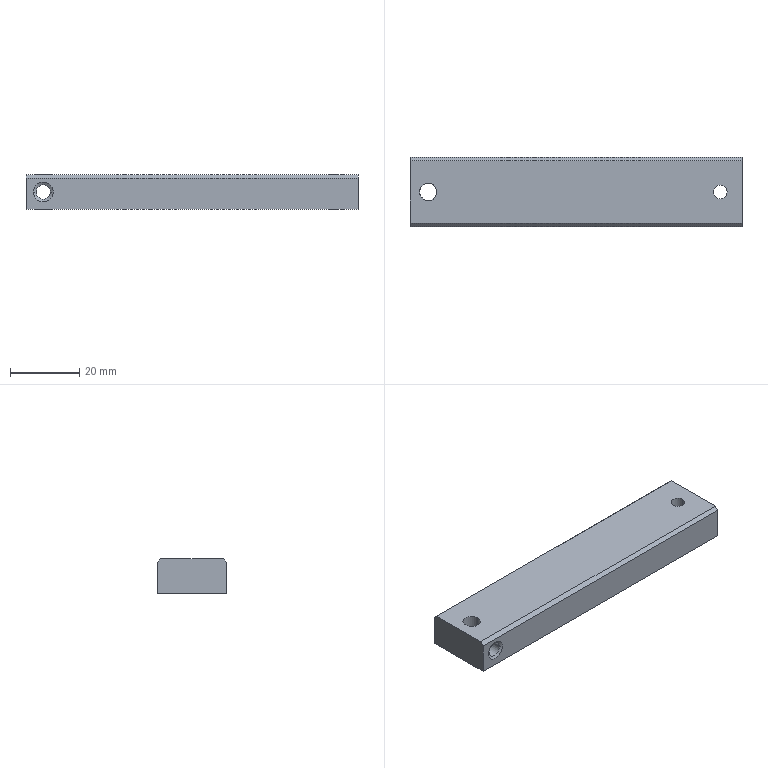Part | NX | 1 solid | 24 faces | box 96 x 20 x 10 mm | volume 18522 mm3 | cylinder 10 | plane 8 | cone 6 | commonest cylinder face diameters 4.2 x4 3.3 x2 4 x2 5 x2
STEP:
#1=CARTESIAN_POINT('',(-48.,-10.,-5.));
#2=VERTEX_POINT('',#1);
#3=CARTESIAN_POINT('',(-48.,10.,-5.));
#4=VERTEX_POINT('',#3);
#5=CARTESIAN_POINT('',(-48.,-10.,-5.));
#6=DIRECTION('',(0.,1.,0.));
#7=VECTOR('',#6,1000.);
#8=LINE('',#5,#7);
#9=EDGE_CURVE('',#2,#4,#8,.T.);
#10=ORIENTED_EDGE('',*,*,#9,.T.);
#11=CARTESIAN_POINT('',(48.,10.,-5.));
#12=VERTEX_POINT('',#11);
#13=CARTESIAN_POINT('',(0.,10.,-5.));
#14=DIRECTION('',(-1.,0.,0.));
#15=VECTOR('',#14,1000.);
#16=LINE('',#13,#15);
#17=EDGE_CURVE('',#12,#4,#16,.T.);
#18=ORIENTED_EDGE('',*,*,#17,.F.);
#19=CARTESIAN_POINT('',(48.,-10.,-5.));
#20=VERTEX_POINT('',#19);
#21=CARTESIAN_POINT('',(48.,0.,-5.));
#22=DIRECTION('',(0.,1.,0.));
#23=VECTOR('',#22,1000.);
#24=LINE('',#21,#23);
#25=EDGE_CURVE('',#20,#12,#24,.T.);
#26=ORIENTED_EDGE('',*,*,#25,.F.);
#27=CARTESIAN_POINT('',(0.,-10.,-5.));
#28=DIRECTION('',(1.,0.,0.));
#29=VECTOR('',#28,1000.);
#30=LINE('',#27,#29);
#31=EDGE_CURVE('',#2,#20,#30,.T.);
#32=ORIENTED_EDGE('',*,*,#31,.F.);
#33=EDGE_LOOP('',(#10,#18,#26,#32));
#34=FACE_BOUND('',#33,.T.);
#35=CARTESIAN_POINT('',(-45.2,0.,-5.));
#36=VERTEX_POINT('',#35);
#37=CARTESIAN_POINT('',(-40.2,0.,-5.));
#38=VERTEX_POINT('',#37);
#39=CARTESIAN_POINT('',(-42.7,0.,-5.));
#40=DIRECTION('',(0.,0.,1.));
#41=DIRECTION('',(-1.,0.,0.));
#42=AXIS2_PLACEMENT_3D('',#39,#40,#41);
#43=CIRCLE('',#42,2.5);
#44=EDGE_CURVE('',#36,#38,#43,.T.);
#45=ORIENTED_EDGE('',*,*,#44,.T.);
#46=CARTESIAN_POINT('',(-42.7,0.,-5.));
#47=DIRECTION('',(0.,0.,1.));
#48=DIRECTION('',(-1.,0.,0.));
#49=AXIS2_PLACEMENT_3D('',#46,#47,#48);
#50=CIRCLE('',#49,2.5);
#51=EDGE_CURVE('',#38,#36,#50,.T.);
#52=ORIENTED_EDGE('',*,*,#51,.T.);
#53=EDGE_LOOP('',(#45,#52));
#54=FACE_BOUND('',#53,.T.);
#55=CARTESIAN_POINT('',(43.7,0.,-5.));
#56=VERTEX_POINT('',#55);
#57=CARTESIAN_POINT('',(39.7,0.,-5.));
#58=VERTEX_POINT('',#57);
#59=CARTESIAN_POINT('',(41.7,0.,-5.));
#60=DIRECTION('',(0.,0.,-1.));
#61=DIRECTION('',(-1.,0.,0.));
#62=AXIS2_PLACEMENT_3D('',#59,#60,#61);
#63=CIRCLE('',#62,2.);
#64=EDGE_CURVE('',#56,#58,#63,.T.);
#65=ORIENTED_EDGE('',*,*,#64,.F.);
#66=CARTESIAN_POINT('',(41.7,0.,-5.));
#67=DIRECTION('',(0.,0.,-1.));
#68=DIRECTION('',(-1.,0.,0.));
#69=AXIS2_PLACEMENT_3D('',#66,#67,#68);
#70=CIRCLE('',#69,2.);
#71=EDGE_CURVE('',#58,#56,#70,.T.);
#72=ORIENTED_EDGE('',*,*,#71,.F.);
#73=EDGE_LOOP('',(#65,#72));
#74=FACE_BOUND('',#73,.T.);
#75=CARTESIAN_POINT('',(0.,0.,-5.));
#76=DIRECTION('',(0.,0.,1.));
#77=DIRECTION('',(1.,0.,0.));
#78=AXIS2_PLACEMENT_3D('',#75,#76,#77);
#79=PLANE('',#78);
#80=ADVANCED_FACE('',(#34,#54,#74),#79,.F.);
#81=ORIENTED_EDGE('',*,*,#9,.F.);
#82=CARTESIAN_POINT('',(-48.,-10.,4.));
#83=VERTEX_POINT('',#82);
#84=CARTESIAN_POINT('',(-48.,-10.,0.));
#85=DIRECTION('',(0.,0.,1.));
#86=VECTOR('',#85,1000.);
#87=LINE('',#84,#86);
#88=EDGE_CURVE('',#2,#83,#87,.T.);
#89=ORIENTED_EDGE('',*,*,#88,.T.);
#90=CARTESIAN_POINT('',(-48.,-9.,5.));
#91=VERTEX_POINT('',#90);
#92=CARTESIAN_POINT('',(-48.,-9.,5.));
#93=DIRECTION('',(0.,-0.7071,-0.7071));
#94=VECTOR('',#93,1000.);
#95=LINE('',#92,#94);
#96=EDGE_CURVE('',#91,#83,#95,.T.);
#97=ORIENTED_EDGE('',*,*,#96,.F.);
#98=CARTESIAN_POINT('',(-48.,9.,5.));
#99=VERTEX_POINT('',#98);
#100=CARTESIAN_POINT('',(-48.,-9.,5.));
#101=DIRECTION('',(0.,1.,0.));
#102=VECTOR('',#101,1000.);
#103=LINE('',#100,#102);
#104=EDGE_CURVE('',#91,#99,#103,.T.);
#105=ORIENTED_EDGE('',*,*,#104,.T.);
#106=CARTESIAN_POINT('',(-48.,10.,4.));
#107=VERTEX_POINT('',#106);
#108=CARTESIAN_POINT('',(-48.,10.,4.));
#109=DIRECTION('',(0.,-0.7071,0.7071));
#110=VECTOR('',#109,1000.);
#111=LINE('',#108,#110);
#112=EDGE_CURVE('',#107,#99,#111,.T.);
#113=ORIENTED_EDGE('',*,*,#112,.F.);
#114=CARTESIAN_POINT('',(-48.,10.,0.));
#115=DIRECTION('',(0.,0.,-1.));
#116=VECTOR('',#115,1000.);
#117=LINE('',#114,#116);
#118=EDGE_CURVE('',#107,#4,#117,.T.);
#119=ORIENTED_EDGE('',*,*,#118,.T.);
#120=EDGE_LOOP('',(#81,#89,#97,#105,#113,#119));
#121=FACE_BOUND('',#120,.T.);
#122=CARTESIAN_POINT('',(-48.,10.,-5.));
#123=DIRECTION('',(-1.,0.,0.));
#124=DIRECTION('',(0.,0.,1.));
#125=AXIS2_PLACEMENT_3D('',#122,#123,#124);
#126=PLANE('',#125);
#127=ADVANCED_FACE('',(#121),#126,.T.);
#128=ORIENTED_EDGE('',*,*,#17,.T.);
#129=ORIENTED_EDGE('',*,*,#118,.F.);
#130=CARTESIAN_POINT('',(48.,10.,4.));
#131=VERTEX_POINT('',#130);
#132=CARTESIAN_POINT('',(0.,10.,4.));
#133=DIRECTION('',(1.,0.,0.));
#134=VECTOR('',#133,1000.);
#135=LINE('',#132,#134);
#136=EDGE_CURVE('',#107,#131,#135,.T.);
#137=ORIENTED_EDGE('',*,*,#136,.T.);
#138=CARTESIAN_POINT('',(48.,10.,0.));
#139=DIRECTION('',(0.,0.,-1.));
#140=VECTOR('',#139,1000.);
#141=LINE('',#138,#140);
#142=EDGE_CURVE('',#131,#12,#141,.T.);
#143=ORIENTED_EDGE('',*,*,#142,.T.);
#144=EDGE_LOOP('',(#128,#129,#137,#143));
#145=FACE_BOUND('',#144,.T.);
#146=CARTESIAN_POINT('',(-40.14,10.,0.));
#147=VERTEX_POINT('',#146);
#148=CARTESIAN_POINT('',(-45.86,10.,0.));
#149=VERTEX_POINT('',#148);
#150=CARTESIAN_POINT('',(-43.,10.,0.));
#151=DIRECTION('',(0.,1.,0.));
#152=DIRECTION('',(1.,0.,0.));
#153=AXIS2_PLACEMENT_3D('',#150,#151,#152);
#154=CIRCLE('',#153,2.86);
#155=EDGE_CURVE('',#147,#149,#154,.T.);
#156=ORIENTED_EDGE('',*,*,#155,.F.);
#157=CARTESIAN_POINT('',(-43.,10.,0.));
#158=DIRECTION('',(0.,1.,0.));
#159=DIRECTION('',(1.,0.,0.));
#160=AXIS2_PLACEMENT_3D('',#157,#158,#159);
#161=CIRCLE('',#160,2.86);
#162=EDGE_CURVE('',#149,#147,#161,.T.);
#163=ORIENTED_EDGE('',*,*,#162,.F.);
#164=EDGE_LOOP('',(#156,#163));
#165=FACE_BOUND('',#164,.T.);
#166=CARTESIAN_POINT('',(48.,10.,-5.));
#167=DIRECTION('',(0.,1.,0.));
#168=DIRECTION('',(1.,0.,0.));
#169=AXIS2_PLACEMENT_3D('',#166,#167,#168);
#170=PLANE('',#169);
#171=ADVANCED_FACE('',(#145,#165),#170,.T.);
#172=ORIENTED_EDGE('',*,*,#25,.T.);
#173=ORIENTED_EDGE('',*,*,#142,.F.);
#174=CARTESIAN_POINT('',(48.,9.,5.));
#175=VERTEX_POINT('',#174);
#176=CARTESIAN_POINT('',(48.,14.,0.));
#177=DIRECTION('',(0.,-0.7071,0.7071));
#178=VECTOR('',#177,1000.);
#179=LINE('',#176,#178);
#180=EDGE_CURVE('',#131,#175,#179,.T.);
#181=ORIENTED_EDGE('',*,*,#180,.T.);
#182=CARTESIAN_POINT('',(48.,-9.,5.));
#183=VERTEX_POINT('',#182);
#184=CARTESIAN_POINT('',(48.,0.,5.));
#185=DIRECTION('',(0.,1.,0.));
#186=VECTOR('',#185,1000.);
#187=LINE('',#184,#186);
#188=EDGE_CURVE('',#183,#175,#187,.T.);
#189=ORIENTED_EDGE('',*,*,#188,.F.);
#190=CARTESIAN_POINT('',(48.,-10.,4.));
#191=VERTEX_POINT('',#190);
#192=CARTESIAN_POINT('',(48.,-14.,0.));
#193=DIRECTION('',(0.,-0.7071,-0.7071));
#194=VECTOR('',#193,1000.);
#195=LINE('',#192,#194);
#196=EDGE_CURVE('',#183,#191,#195,.T.);
#197=ORIENTED_EDGE('',*,*,#196,.T.);
#198=CARTESIAN_POINT('',(48.,-10.,0.));
#199=DIRECTION('',(0.,0.,1.));
#200=VECTOR('',#199,1000.);
#201=LINE('',#198,#200);
#202=EDGE_CURVE('',#20,#191,#201,.T.);
#203=ORIENTED_EDGE('',*,*,#202,.F.);
#204=EDGE_LOOP('',(#172,#173,#181,#189,#197,#203));
#205=FACE_BOUND('',#204,.T.);
#206=CARTESIAN_POINT('',(48.,-2.315,0.));
#207=VERTEX_POINT('',#206);
#208=CARTESIAN_POINT('',(48.,2.315,0.));
#209=VERTEX_POINT('',#208);
#210=CARTESIAN_POINT('',(48.,0.,0.));
#211=DIRECTION('',(1.,0.,0.));
#212=DIRECTION('',(0.,-1.,0.));
#213=AXIS2_PLACEMENT_3D('',#210,#211,#212);
#214=CIRCLE('',#213,2.315);
#215=EDGE_CURVE('',#207,#209,#214,.T.);
#216=ORIENTED_EDGE('',*,*,#215,.F.);
#217=CARTESIAN_POINT('',(48.,0.,0.));
#218=DIRECTION('',(1.,0.,0.));
#219=DIRECTION('',(0.,-1.,0.));
#220=AXIS2_PLACEMENT_3D('',#217,#218,#219);
#221=CIRCLE('',#220,2.315);
#222=EDGE_CURVE('',#209,#207,#221,.T.);
#223=ORIENTED_EDGE('',*,*,#222,.F.);
#224=EDGE_LOOP('',(#216,#223));
#225=FACE_BOUND('',#224,.T.);
#226=CARTESIAN_POINT('',(48.,-10.,-5.));
#227=DIRECTION('',(1.,0.,0.));
#228=DIRECTION('',(0.,1.,0.));
#229=AXIS2_PLACEMENT_3D('',#226,#227,#228);
#230=PLANE('',#229);
#231=ADVANCED_FACE('',(#205,#225),#230,.T.);
#232=ORIENTED_EDGE('',*,*,#31,.T.);
#233=ORIENTED_EDGE('',*,*,#202,.T.);
#234=CARTESIAN_POINT('',(0.,-10.,4.));
#235=DIRECTION('',(-1.,0.,0.));
#236=VECTOR('',#235,1000.);
#237=LINE('',#234,#236);
#238=EDGE_CURVE('',#191,#83,#237,.T.);
#239=ORIENTED_EDGE('',*,*,#238,.T.);
#240=ORIENTED_EDGE('',*,*,#88,.F.);
#241=EDGE_LOOP('',(#232,#233,#239,#240));
#242=FACE_BOUND('',#241,.T.);
#243=CARTESIAN_POINT('',(-40.14,-10.,0.));
#244=VERTEX_POINT('',#243);
#245=CARTESIAN_POINT('',(-45.86,-10.,0.));
#246=VERTEX_POINT('',#245);
#247=CARTESIAN_POINT('',(-43.,-10.,0.));
#248=DIRECTION('',(0.,-1.,0.));
#249=DIRECTION('',(-1.,0.,0.));
#250=AXIS2_PLACEMENT_3D('',#247,#248,#249);
#251=CIRCLE('',#250,2.86);
#252=EDGE_CURVE('',#244,#246,#251,.T.);
#253=ORIENTED_EDGE('',*,*,#252,.F.);
#254=CARTESIAN_POINT('',(-43.,-10.,0.));
#255=DIRECTION('',(0.,-1.,0.));
#256=DIRECTION('',(-1.,0.,0.));
#257=AXIS2_PLACEMENT_3D('',#254,#255,#256);
#258=CIRCLE('',#257,2.86);
#259=EDGE_CURVE('',#246,#244,#258,.T.);
#260=ORIENTED_EDGE('',*,*,#259,.F.);
#261=EDGE_LOOP('',(#253,#260));
#262=FACE_BOUND('',#261,.T.);
#263=CARTESIAN_POINT('',(-48.,-10.,-5.));
#264=DIRECTION('',(0.,-1.,0.));
#265=DIRECTION('',(0.,0.,-1.));
#266=AXIS2_PLACEMENT_3D('',#263,#264,#265);
#267=PLANE('',#266);
#268=ADVANCED_FACE('',(#242,#262),#267,.T.);
#269=CARTESIAN_POINT('',(48.,-9.,5.));
#270=DIRECTION('',(-1.,0.,0.));
#271=VECTOR('',#270,1000.);
#272=LINE('',#269,#271);
#273=EDGE_CURVE('',#183,#91,#272,.T.);
#274=ORIENTED_EDGE('',*,*,#273,.T.);
#275=ORIENTED_EDGE('',*,*,#96,.T.);
#276=ORIENTED_EDGE('',*,*,#238,.F.);
#277=ORIENTED_EDGE('',*,*,#196,.F.);
#278=EDGE_LOOP('',(#274,#275,#276,#277));
#279=FACE_BOUND('',#278,.T.);
#280=CARTESIAN_POINT('',(-48.,-9.,5.));
#281=DIRECTION('',(0.,0.7071,-0.7071));
#282=DIRECTION('',(-1.,0.,0.));
#283=AXIS2_PLACEMENT_3D('',#280,#281,#282);
#284=PLANE('',#283);
#285=ADVANCED_FACE('',(#279),#284,.F.);
#286=ORIENTED_EDGE('',*,*,#104,.F.);
#287=ORIENTED_EDGE('',*,*,#273,.F.);
#288=ORIENTED_EDGE('',*,*,#188,.T.);
#289=CARTESIAN_POINT('',(-48.,9.,5.));
#290=DIRECTION('',(1.,0.,0.));
#291=VECTOR('',#290,1000.);
#292=LINE('',#289,#291);
#293=EDGE_CURVE('',#99,#175,#292,.T.);
#294=ORIENTED_EDGE('',*,*,#293,.F.);
#295=EDGE_LOOP('',(#286,#287,#288,#294));
#296=FACE_BOUND('',#295,.T.);
#297=CARTESIAN_POINT('',(-40.2,0.,5.));
#298=VERTEX_POINT('',#297);
#299=CARTESIAN_POINT('',(-45.2,0.,5.));
#300=VERTEX_POINT('',#299);
#301=CARTESIAN_POINT('',(-42.7,0.,5.));
#302=DIRECTION('',(0.,0.,1.));
#303=DIRECTION('',(-1.,0.,0.));
#304=AXIS2_PLACEMENT_3D('',#301,#302,#303);
#305=CIRCLE('',#304,2.5);
#306=EDGE_CURVE('',#298,#300,#305,.T.);
#307=ORIENTED_EDGE('',*,*,#306,.F.);
#308=CARTESIAN_POINT('',(-42.7,0.,5.));
#309=DIRECTION('',(0.,0.,1.));
#310=DIRECTION('',(-1.,0.,0.));
#311=AXIS2_PLACEMENT_3D('',#308,#309,#310);
#312=CIRCLE('',#311,2.5);
#313=EDGE_CURVE('',#300,#298,#312,.T.);
#314=ORIENTED_EDGE('',*,*,#313,.F.);
#315=EDGE_LOOP('',(#307,#314));
#316=FACE_BOUND('',#315,.T.);
#317=CARTESIAN_POINT('',(39.7,0.,5.));
#318=VERTEX_POINT('',#317);
#319=CARTESIAN_POINT('',(43.7,0.,5.));
#320=VERTEX_POINT('',#319);
#321=CARTESIAN_POINT('',(41.7,0.,5.));
#322=DIRECTION('',(0.,0.,-1.));
#323=DIRECTION('',(-1.,0.,0.));
#324=AXIS2_PLACEMENT_3D('',#321,#322,#323);
#325=CIRCLE('',#324,2.);
#326=EDGE_CURVE('',#318,#320,#325,.T.);
#327=ORIENTED_EDGE('',*,*,#326,.T.);
#328=CARTESIAN_POINT('',(41.7,0.,5.));
#329=DIRECTION('',(0.,0.,-1.));
#330=DIRECTION('',(-1.,0.,0.));
#331=AXIS2_PLACEMENT_3D('',#328,#329,#330);
#332=CIRCLE('',#331,2.);
#333=EDGE_CURVE('',#320,#318,#332,.T.);
#334=ORIENTED_EDGE('',*,*,#333,.T.);
#335=EDGE_LOOP('',(#327,#334));
#336=FACE_BOUND('',#335,.T.);
#337=CARTESIAN_POINT('',(0.,0.,5.));
#338=DIRECTION('',(0.,0.,1.));
#339=DIRECTION('',(1.,0.,0.));
#340=AXIS2_PLACEMENT_3D('',#337,#338,#339);
#341=PLANE('',#340);
#342=ADVANCED_FACE('',(#296,#316,#336),#341,.T.);
#343=ORIENTED_EDGE('',*,*,#293,.T.);
#344=ORIENTED_EDGE('',*,*,#180,.F.);
#345=ORIENTED_EDGE('',*,*,#136,.F.);
#346=ORIENTED_EDGE('',*,*,#112,.T.);
#347=EDGE_LOOP('',(#343,#344,#345,#346));
#348=FACE_BOUND('',#347,.T.);
#349=CARTESIAN_POINT('',(48.,9.,5.));
#350=DIRECTION('',(0.,-0.7071,-0.7071));
#351=DIRECTION('',(0.,-0.7071,0.7071));
#352=AXIS2_PLACEMENT_3D('',#349,#350,#351);
#353=PLANE('',#352);
#354=ADVANCED_FACE('',(#348),#353,.F.);
#355=ORIENTED_EDGE('',*,*,#44,.F.);
#356=CARTESIAN_POINT('',(-45.2,0.,-6.55));
#357=DIRECTION('',(0.,0.,1.));
#358=VECTOR('',#357,1000.);
#359=LINE('',#356,#358);
#360=EDGE_CURVE('',#300,#36,#359,.F.);
#361=ORIENTED_EDGE('',*,*,#360,.F.);
#362=ORIENTED_EDGE('',*,*,#313,.T.);
#363=CARTESIAN_POINT('',(-40.2,0.,-6.55));
#364=DIRECTION('',(0.,0.,1.));
#365=VECTOR('',#364,1000.);
#366=LINE('',#363,#365);
#367=EDGE_CURVE('',#298,#38,#366,.F.);
#368=ORIENTED_EDGE('',*,*,#367,.T.);
#369=EDGE_LOOP('',(#355,#361,#362,#368));
#370=FACE_BOUND('',#369,.T.);
#371=CARTESIAN_POINT('',(-40.9,-1.735,0.));
#372=VERTEX_POINT('',#371);
#373=CARTESIAN_POINT('',(-45.1,-0.7,0.));
#374=VERTEX_POINT('',#373);
#375=CARTESIAN_POINT('',(-40.9,-1.735,0.));
#376=CARTESIAN_POINT('',(-40.9,-1.735,0.5723));
#377=CARTESIAN_POINT('',(-41.28,-2.154,1.427));
#378=CARTESIAN_POINT('',(-42.274,-2.52,2.044));
#379=CARTESIAN_POINT('',(-43.235,-2.492,2.143));
#380=CARTESIAN_POINT('',(-43.941,-2.22,1.932));
#381=CARTESIAN_POINT('',(-44.527,-1.744,1.488));
#382=CARTESIAN_POINT('',(-44.808,-1.354,1.083));
#383=CARTESIAN_POINT('',(-44.951,-1.106,0.814));
#384=CARTESIAN_POINT('',(-45.089,-0.7549,0.3321));
#385=CARTESIAN_POINT('',(-45.1,-0.7002,0.1078));
#386=CARTESIAN_POINT('',(-45.1,-0.7,0.));
#387=B_SPLINE_CURVE_WITH_KNOTS('',3,(#375,#376,#377,#378,#379,#380,#381,#382,#383,#384,#385,#386),.UNSPECIFIED.,.F.,.F.,(4,1,1,1,1,1,1,1,1,4),(0.,0.25,0.375,0.5,0.625,0.75,0.8125,0.875,0.9375,1.),.UNSPECIFIED.);
#388=EDGE_CURVE('',#372,#374,#387,.T.);
#389=ORIENTED_EDGE('',*,*,#388,.T.);
#390=CARTESIAN_POINT('',(-45.1,-0.7,0.));
#391=CARTESIAN_POINT('',(-45.1,-0.7002,-0.1303));
#392=CARTESIAN_POINT('',(-45.079,-0.7833,-0.3831));
#393=CARTESIAN_POINT('',(-44.913,-1.198,-0.9315));
#394=CARTESIAN_POINT('',(-44.646,-1.636,-1.378));
#395=CARTESIAN_POINT('',(-43.941,-2.224,-1.938));
#396=CARTESIAN_POINT('',(-43.235,-2.491,-2.141));
#397=CARTESIAN_POINT('',(-42.273,-2.52,-2.044));
#398=CARTESIAN_POINT('',(-41.281,-2.155,-1.427));
#399=CARTESIAN_POINT('',(-40.9,-1.735,-0.5728));
#400=CARTESIAN_POINT('',(-40.9,-1.735,0.));
#401=B_SPLINE_CURVE_WITH_KNOTS('',3,(#390,#391,#392,#393,#394,#395,#396,#397,#398,#399,#400),.UNSPECIFIED.,.F.,.F.,(4,1,1,1,1,1,1,1,4),(0.,0.0625,0.125,0.25,0.375,0.5,0.625,0.75,1.),.UNSPECIFIED.);
#402=EDGE_CURVE('',#374,#372,#401,.T.);
#403=ORIENTED_EDGE('',*,*,#402,.T.);
#404=EDGE_LOOP('',(#389,#403));
#405=FACE_BOUND('',#404,.T.);
#406=CARTESIAN_POINT('',(-42.7,0.,-6.55));
#407=DIRECTION('',(0.,0.,1.));
#408=DIRECTION('',(-1.,0.,0.));
#409=AXIS2_PLACEMENT_3D('',#406,#407,#408);
#410=CYLINDRICAL_SURFACE('',#409,2.5);
#411=ADVANCED_FACE('',(#370,#405),#410,.F.);
#412=ORIENTED_EDGE('',*,*,#252,.T.);
#413=CARTESIAN_POINT('',(-45.1,-9.561,0.));
#414=VERTEX_POINT('',#413);
#415=CARTESIAN_POINT('',(-45.1,-9.561,0.));
#416=DIRECTION('',(-0.866,-0.5,0.));
#417=VECTOR('',#416,1000.);
#418=LINE('',#415,#417);
#419=EDGE_CURVE('',#246,#414,#418,.F.);
#420=ORIENTED_EDGE('',*,*,#419,.T.);
#421=CARTESIAN_POINT('',(-40.9,-9.561,0.));
#422=VERTEX_POINT('',#421);
#423=CARTESIAN_POINT('',(-43.,-9.561,0.));
#424=DIRECTION('',(0.,-1.,0.));
#425=DIRECTION('',(-1.,0.,0.));
#426=AXIS2_PLACEMENT_3D('',#423,#424,#425);
#427=CIRCLE('',#426,2.1);
#428=EDGE_CURVE('',#422,#414,#427,.T.);
#429=ORIENTED_EDGE('',*,*,#428,.F.);
#430=CARTESIAN_POINT('',(-40.9,-9.561,0.));
#431=DIRECTION('',(0.866,-0.5,0.));
#432=VECTOR('',#431,1000.);
#433=LINE('',#430,#432);
#434=EDGE_CURVE('',#244,#422,#433,.F.);
#435=ORIENTED_EDGE('',*,*,#434,.F.);
#436=EDGE_LOOP('',(#412,#420,#429,#435));
#437=FACE_BOUND('',#436,.T.);
#438=CARTESIAN_POINT('',(-43.,-9.561,0.));
#439=DIRECTION('',(0.,-1.,0.));
#440=DIRECTION('',(-1.,0.,0.));
#441=AXIS2_PLACEMENT_3D('',#438,#439,#440);
#442=CONICAL_SURFACE('',#441,2.1,1.047);
#443=ADVANCED_FACE('',(#437),#442,.F.);
#444=ORIENTED_EDGE('',*,*,#155,.T.);
#445=CARTESIAN_POINT('',(-45.1,9.561,0.));
#446=VERTEX_POINT('',#445);
#447=CARTESIAN_POINT('',(-45.1,9.561,0.));
#448=DIRECTION('',(-0.866,0.5,0.));
#449=VECTOR('',#448,1000.);
#450=LINE('',#447,#449);
#451=EDGE_CURVE('',#149,#446,#450,.F.);
#452=ORIENTED_EDGE('',*,*,#451,.T.);
#453=CARTESIAN_POINT('',(-40.9,9.561,0.));
#454=VERTEX_POINT('',#453);
#455=CARTESIAN_POINT('',(-43.,9.561,0.));
#456=DIRECTION('',(0.,1.,0.));
#457=DIRECTION('',(1.,0.,0.));
#458=AXIS2_PLACEMENT_3D('',#455,#456,#457);
#459=CIRCLE('',#458,2.1);
#460=EDGE_CURVE('',#454,#446,#459,.T.);
#461=ORIENTED_EDGE('',*,*,#460,.F.);
#462=CARTESIAN_POINT('',(-40.9,9.561,0.));
#463=DIRECTION('',(0.866,0.5,0.));
#464=VECTOR('',#463,1000.);
#465=LINE('',#462,#464);
#466=EDGE_CURVE('',#147,#454,#465,.F.);
#467=ORIENTED_EDGE('',*,*,#466,.F.);
#468=EDGE_LOOP('',(#444,#452,#461,#467));
#469=FACE_BOUND('',#468,.T.);
#470=CARTESIAN_POINT('',(-43.,9.561,0.));
#471=DIRECTION('',(0.,1.,0.));
#472=DIRECTION('',(1.,0.,0.));
#473=AXIS2_PLACEMENT_3D('',#470,#471,#472);
#474=CONICAL_SURFACE('',#473,2.1,1.047);
#475=ADVANCED_FACE('',(#469),#474,.F.);
#476=ORIENTED_EDGE('',*,*,#326,.F.);
#477=CARTESIAN_POINT('',(39.7,0.,5.));
#478=DIRECTION('',(0.,0.,-1.));
#479=VECTOR('',#478,1000.);
#480=LINE('',#477,#479);
#481=EDGE_CURVE('',#58,#318,#480,.F.);
#482=ORIENTED_EDGE('',*,*,#481,.F.);
#483=ORIENTED_EDGE('',*,*,#71,.T.);
#484=CARTESIAN_POINT('',(43.7,0.,-1.65));
#485=VERTEX_POINT('',#484);
#486=CARTESIAN_POINT('',(43.7,0.,5.));
#487=DIRECTION('',(0.,0.,-1.));
#488=VECTOR('',#487,1000.);
#489=LINE('',#486,#488);
#490=EDGE_CURVE('',#485,#56,#489,.T.);
#491=ORIENTED_EDGE('',*,*,#490,.F.);
#492=CARTESIAN_POINT('',(42.83,1.65,0.));
#493=VERTEX_POINT('',#492);
#494=CARTESIAN_POINT('',(43.7,0.,-1.65));
#495=CARTESIAN_POINT('',(43.7,0.4508,-1.65));
#496=CARTESIAN_POINT('',(43.439,1.102,-1.339));
#497=CARTESIAN_POINT('',(42.983,1.549,-0.6815));
#498=CARTESIAN_POINT('',(42.83,1.65,-0.2103));
#499=CARTESIAN_POINT('',(42.83,1.65,0.));
#500=B_SPLINE_CURVE_WITH_KNOTS('',3,(#494,#495,#496,#497,#498,#499),.UNSPECIFIED.,.F.,.F.,(4,1,1,4),(0.,0.5,0.75,1.),.UNSPECIFIED.);
#501=EDGE_CURVE('',#485,#493,#500,.T.);
#502=ORIENTED_EDGE('',*,*,#501,.T.);
#503=CARTESIAN_POINT('',(43.7,0.,1.65));
#504=VERTEX_POINT('',#503);
#505=CARTESIAN_POINT('',(42.83,1.65,0.));
#506=CARTESIAN_POINT('',(42.83,1.65,0.2102));
#507=CARTESIAN_POINT('',(42.983,1.549,0.6815));
#508=CARTESIAN_POINT('',(43.439,1.102,1.339));
#509=CARTESIAN_POINT('',(43.7,0.451,1.65));
#510=CARTESIAN_POINT('',(43.7,0.,1.65));
#511=B_SPLINE_CURVE_WITH_KNOTS('',3,(#505,#506,#507,#508,#509,#510),.UNSPECIFIED.,.F.,.F.,(4,1,1,4),(0.,0.25,0.5,1.),.UNSPECIFIED.);
#512=EDGE_CURVE('',#493,#504,#511,.T.);
#513=ORIENTED_EDGE('',*,*,#512,.T.);
#514=CARTESIAN_POINT('',(43.7,0.,5.));
#515=DIRECTION('',(0.,0.,-1.));
#516=VECTOR('',#515,1000.);
#517=LINE('',#514,#516);
#518=EDGE_CURVE('',#504,#320,#517,.F.);
#519=ORIENTED_EDGE('',*,*,#518,.T.);
#520=EDGE_LOOP('',(#476,#482,#483,#491,#502,#513,#519));
#521=FACE_BOUND('',#520,.T.);
#522=CARTESIAN_POINT('',(41.7,0.,5.));
#523=DIRECTION('',(0.,0.,-1.));
#524=DIRECTION('',(-1.,0.,0.));
#525=AXIS2_PLACEMENT_3D('',#522,#523,#524);
#526=CYLINDRICAL_SURFACE('',#525,2.);
#527=ADVANCED_FACE('',(#521),#526,.F.);
#528=CARTESIAN_POINT('',(-43.,9.561,0.));
#529=DIRECTION('',(0.,1.,0.));
#530=DIRECTION('',(1.,0.,0.));
#531=AXIS2_PLACEMENT_3D('',#528,#529,#530);
#532=CIRCLE('',#531,2.1);
#533=EDGE_CURVE('',#446,#454,#532,.T.);
#534=ORIENTED_EDGE('',*,*,#533,.T.);
#535=CARTESIAN_POINT('',(-40.9,1.735,0.));
#536=VERTEX_POINT('',#535);
#537=CARTESIAN_POINT('',(-40.9,10.,0.));
#538=DIRECTION('',(0.,1.,0.));
#539=VECTOR('',#538,1000.);
#540=LINE('',#537,#539);
#541=EDGE_CURVE('',#536,#454,#540,.T.);
#542=ORIENTED_EDGE('',*,*,#541,.F.);
#543=CARTESIAN_POINT('',(-45.1,0.7,0.));
#544=VERTEX_POINT('',#543);
#545=CARTESIAN_POINT('',(-40.9,1.735,0.));
#546=CARTESIAN_POINT('',(-40.9,1.735,0.129));
#547=CARTESIAN_POINT('',(-40.915,1.756,0.3881));
#548=CARTESIAN_POINT('',(-41.063,1.891,0.8278));
#549=CARTESIAN_POINT('',(-41.152,1.964,1.001));
#550=CARTESIAN_POINT('',(-41.282,2.063,1.221));
#551=CARTESIAN_POINT('',(-41.473,2.179,1.445));
#552=CARTESIAN_POINT('',(-41.546,2.219,1.519));
#553=CARTESIAN_POINT('',(-41.76,2.319,1.702));
#554=CARTESIAN_POINT('',(-42.007,2.405,1.857));
#555=CARTESIAN_POINT('',(-42.406,2.51,2.05));
#556=CARTESIAN_POINT('',(-43.076,2.501,2.132));
#557=CARTESIAN_POINT('',(-43.593,2.349,2.03));
#558=CARTESIAN_POINT('',(-44.022,2.134,1.848));
#559=CARTESIAN_POINT('',(-44.281,1.949,1.679));
#560=CARTESIAN_POINT('',(-44.56,1.678,1.416));
#561=CARTESIAN_POINT('',(-44.68,1.527,1.262));
#562=CARTESIAN_POINT('',(-44.787,1.384,1.114));
#563=CARTESIAN_POINT('',(-44.923,1.148,0.8493));
#564=CARTESIAN_POINT('',(-44.938,1.116,0.8146));
#565=CARTESIAN_POINT('',(-45.027,0.9205,0.5631));
#566=CARTESIAN_POINT('',(-45.066,0.8079,0.3979));
#567=CARTESIAN_POINT('',(-45.1,0.7,0.1272));
#568=CARTESIAN_POINT('',(-45.1,0.7,0.));
#569=B_SPLINE_CURVE_WITH_KNOTS('',3,(#545,#546,#547,#548,#549,#550,#551,#552,#553,#554,#555,#556,#557,#558,#559,#560,#561,#562,#563,#564,#565,#566,#567,#568),.UNSPECIFIED.,.F.,.F.,(4,1,1,1,1,1,1,1,1,1,1,1,1,1,1,1,1,1,1,1,1,4),(0.,0.0625,0.125,0.1562,0.1875,0.2188,0.25,0.2812,0.3125,0.375,0.5,0.5625,0.625,0.6875,0.75,0.7812,0.8125,0.8438,0.875,0.9062,0.9375,1.),.UNSPECIFIED.);
#570=EDGE_CURVE('',#536,#544,#569,.T.);
#571=ORIENTED_EDGE('',*,*,#570,.T.);
#572=CARTESIAN_POINT('',(-45.1,10.,0.));
#573=DIRECTION('',(0.,1.,0.));
#574=VECTOR('',#573,1000.);
#575=LINE('',#572,#574);
#576=EDGE_CURVE('',#544,#446,#575,.T.);
#577=ORIENTED_EDGE('',*,*,#576,.T.);
#578=EDGE_LOOP('',(#534,#542,#571,#577));
#579=FACE_BOUND('',#578,.T.);
#580=CARTESIAN_POINT('',(-43.,10.,0.));
#581=DIRECTION('',(0.,1.,0.));
#582=DIRECTION('',(1.,0.,0.));
#583=AXIS2_PLACEMENT_3D('',#580,#581,#582);
#584=CYLINDRICAL_SURFACE('',#583,2.1);
#585=ADVANCED_FACE('',(#579),#584,.F.);
#586=ORIENTED_EDGE('',*,*,#388,.F.);
#587=CARTESIAN_POINT('',(-40.9,-10.,0.));
#588=DIRECTION('',(0.,-1.,0.));
#589=VECTOR('',#588,1000.);
#590=LINE('',#587,#589);
#591=EDGE_CURVE('',#372,#422,#590,.T.);
#592=ORIENTED_EDGE('',*,*,#591,.T.);
#593=ORIENTED_EDGE('',*,*,#428,.T.);
#594=CARTESIAN_POINT('',(-45.1,-10.,0.));
#595=DIRECTION('',(0.,-1.,0.));
#596=VECTOR('',#595,1000.);
#597=LINE('',#594,#596);
#598=EDGE_CURVE('',#374,#414,#597,.T.);
#599=ORIENTED_EDGE('',*,*,#598,.F.);
#600=EDGE_LOOP('',(#586,#592,#593,#599));
#601=FACE_BOUND('',#600,.T.);
#602=CARTESIAN_POINT('',(-43.,-10.,0.));
#603=DIRECTION('',(0.,-1.,0.));
#604=DIRECTION('',(-1.,0.,0.));
#605=AXIS2_PLACEMENT_3D('',#602,#603,#604);
#606=CYLINDRICAL_SURFACE('',#605,2.1);
#607=ADVANCED_FACE('',(#601),#606,.F.);
#608=CARTESIAN_POINT('',(42.83,-1.65,0.));
#609=VERTEX_POINT('',#608);
#610=CARTESIAN_POINT('',(43.7,0.,-1.65));
#611=CARTESIAN_POINT('',(43.7,-0.2195,-1.65));
#612=CARTESIAN_POINT('',(43.625,-0.5988,-1.558));
#613=CARTESIAN_POINT('',(43.489,-0.9084,-1.39));
#614=CARTESIAN_POINT('',(43.256,-1.288,-1.076));
#615=CARTESIAN_POINT('',(42.987,-1.542,-0.6894));
#616=CARTESIAN_POINT('',(42.83,-1.65,-0.2066));
#617=CARTESIAN_POINT('',(42.83,-1.65,0.));
#618=B_SPLINE_CURVE_WITH_KNOTS('',3,(#610,#611,#612,#613,#614,#615,#616,#617),.UNSPECIFIED.,.F.,.F.,(4,1,1,1,1,4),(0.,0.25,0.375,0.5,0.75,1.),.UNSPECIFIED.);
#619=EDGE_CURVE('',#609,#485,#618,.F.);
#620=ORIENTED_EDGE('',*,*,#619,.F.);
#621=CARTESIAN_POINT('',(47.616,-1.65,0.));
#622=VERTEX_POINT('',#621);
#623=CARTESIAN_POINT('',(48.,-1.65,0.));
#624=DIRECTION('',(1.,0.,0.));
#625=VECTOR('',#624,1000.);
#626=LINE('',#623,#625);
#627=EDGE_CURVE('',#622,#609,#626,.F.);
#628=ORIENTED_EDGE('',*,*,#627,.F.);
#629=CARTESIAN_POINT('',(47.616,1.65,0.));
#630=VERTEX_POINT('',#629);
#631=CARTESIAN_POINT('',(47.616,0.,0.));
#632=DIRECTION('',(1.,0.,0.));
#633=DIRECTION('',(0.,-1.,0.));
#634=AXIS2_PLACEMENT_3D('',#631,#632,#633);
#635=CIRCLE('',#634,1.65);
#636=EDGE_CURVE('',#622,#630,#635,.T.);
#637=ORIENTED_EDGE('',*,*,#636,.T.);
#638=CARTESIAN_POINT('',(48.,1.65,0.));
#639=DIRECTION('',(1.,0.,0.));
#640=VECTOR('',#639,1000.);
#641=LINE('',#638,#640);
#642=EDGE_CURVE('',#630,#493,#641,.F.);
#643=ORIENTED_EDGE('',*,*,#642,.T.);
#644=ORIENTED_EDGE('',*,*,#501,.F.);
#645=EDGE_LOOP('',(#620,#628,#637,#643,#644));
#646=FACE_BOUND('',#645,.T.);
#647=CARTESIAN_POINT('',(48.,0.,0.));
#648=DIRECTION('',(1.,0.,0.));
#649=DIRECTION('',(0.,-1.,0.));
#650=AXIS2_PLACEMENT_3D('',#647,#648,#649);
#651=CYLINDRICAL_SURFACE('',#650,1.65);
#652=ADVANCED_FACE('',(#646),#651,.F.);
#653=ORIENTED_EDGE('',*,*,#636,.F.);
#654=CARTESIAN_POINT('',(47.616,-1.65,0.));
#655=DIRECTION('',(0.5,-0.866,0.));
#656=VECTOR('',#655,1000.);
#657=LINE('',#654,#656);
#658=EDGE_CURVE('',#207,#622,#657,.F.);
#659=ORIENTED_EDGE('',*,*,#658,.F.);
#660=ORIENTED_EDGE('',*,*,#215,.T.);
#661=CARTESIAN_POINT('',(47.616,1.65,0.));
#662=DIRECTION('',(0.5,0.866,0.));
#663=VECTOR('',#662,1000.);
#664=LINE('',#661,#663);
#665=EDGE_CURVE('',#209,#630,#664,.F.);
#666=ORIENTED_EDGE('',*,*,#665,.T.);
#667=EDGE_LOOP('',(#653,#659,#660,#666));
#668=FACE_BOUND('',#667,.T.);
#669=CARTESIAN_POINT('',(47.616,0.,0.));
#670=DIRECTION('',(1.,0.,0.));
#671=DIRECTION('',(0.,-1.,0.));
#672=AXIS2_PLACEMENT_3D('',#669,#670,#671);
#673=CONICAL_SURFACE('',#672,1.65,1.047);
#674=ADVANCED_FACE('',(#668),#673,.F.);
#675=ORIENTED_EDGE('',*,*,#533,.F.);
#676=ORIENTED_EDGE('',*,*,#451,.F.);
#677=ORIENTED_EDGE('',*,*,#162,.T.);
#678=ORIENTED_EDGE('',*,*,#466,.T.);
#679=EDGE_LOOP('',(#675,#676,#677,#678));
#680=FACE_BOUND('',#679,.T.);
#681=CARTESIAN_POINT('',(-43.,9.561,0.));
#682=DIRECTION('',(0.,1.,0.));
#683=DIRECTION('',(1.,0.,0.));
#684=AXIS2_PLACEMENT_3D('',#681,#682,#683);
#685=CONICAL_SURFACE('',#684,2.1,1.047);
#686=ADVANCED_FACE('',(#680),#685,.F.);
#687=ORIENTED_EDGE('',*,*,#627,.T.);
#688=CARTESIAN_POINT('',(42.83,-1.65,0.));
#689=CARTESIAN_POINT('',(42.83,-1.65,0.1921));
#690=CARTESIAN_POINT('',(42.983,-1.548,0.6897));
#691=CARTESIAN_POINT('',(43.439,-1.105,1.335));
#692=CARTESIAN_POINT('',(43.7,-0.4391,1.65));
#693=CARTESIAN_POINT('',(43.7,0.,1.65));
#694=B_SPLINE_CURVE_WITH_KNOTS('',3,(#688,#689,#690,#691,#692,#693),.UNSPECIFIED.,.F.,.F.,(4,1,1,4),(0.,0.25,0.5,1.),.UNSPECIFIED.);
#695=EDGE_CURVE('',#504,#609,#694,.F.);
#696=ORIENTED_EDGE('',*,*,#695,.F.);
#697=ORIENTED_EDGE('',*,*,#512,.F.);
#698=ORIENTED_EDGE('',*,*,#642,.F.);
#699=CARTESIAN_POINT('',(47.616,0.,0.));
#700=DIRECTION('',(1.,0.,0.));
#701=DIRECTION('',(0.,-1.,0.));
#702=AXIS2_PLACEMENT_3D('',#699,#700,#701);
#703=CIRCLE('',#702,1.65);
#704=EDGE_CURVE('',#630,#622,#703,.T.);
#705=ORIENTED_EDGE('',*,*,#704,.T.);
#706=EDGE_LOOP('',(#687,#696,#697,#698,#705));
#707=FACE_BOUND('',#706,.T.);
#708=CARTESIAN_POINT('',(48.,0.,0.));
#709=DIRECTION('',(1.,0.,0.));
#710=DIRECTION('',(0.,-1.,0.));
#711=AXIS2_PLACEMENT_3D('',#708,#709,#710);
#712=CYLINDRICAL_SURFACE('',#711,1.65);
#713=ADVANCED_FACE('',(#707),#712,.F.);
#714=CARTESIAN_POINT('',(-43.,-9.561,0.));
#715=DIRECTION('',(0.,-1.,0.));
#716=DIRECTION('',(-1.,0.,0.));
#717=AXIS2_PLACEMENT_3D('',#714,#715,#716);
#718=CIRCLE('',#717,2.1);
#719=EDGE_CURVE('',#414,#422,#718,.T.);
#720=ORIENTED_EDGE('',*,*,#719,.F.);
#721=ORIENTED_EDGE('',*,*,#419,.F.);
#722=ORIENTED_EDGE('',*,*,#259,.T.);
#723=ORIENTED_EDGE('',*,*,#434,.T.);
#724=EDGE_LOOP('',(#720,#721,#722,#723));
#725=FACE_BOUND('',#724,.T.);
#726=CARTESIAN_POINT('',(-43.,-9.561,0.));
#727=DIRECTION('',(0.,-1.,0.));
#728=DIRECTION('',(-1.,0.,0.));
#729=AXIS2_PLACEMENT_3D('',#726,#727,#728);
#730=CONICAL_SURFACE('',#729,2.1,1.047);
#731=ADVANCED_FACE('',(#725),#730,.F.);
#732=ORIENTED_EDGE('',*,*,#64,.T.);
#733=ORIENTED_EDGE('',*,*,#481,.T.);
#734=ORIENTED_EDGE('',*,*,#333,.F.);
#735=ORIENTED_EDGE('',*,*,#518,.F.);
#736=ORIENTED_EDGE('',*,*,#695,.T.);
#737=ORIENTED_EDGE('',*,*,#619,.T.);
#738=ORIENTED_EDGE('',*,*,#490,.T.);
#739=EDGE_LOOP('',(#732,#733,#734,#735,#736,#737,#738));
#740=FACE_BOUND('',#739,.T.);
#741=CARTESIAN_POINT('',(41.7,0.,5.));
#742=DIRECTION('',(0.,0.,-1.));
#743=DIRECTION('',(-1.,0.,0.));
#744=AXIS2_PLACEMENT_3D('',#741,#742,#743);
#745=CYLINDRICAL_SURFACE('',#744,2.);
#746=ADVANCED_FACE('',(#740),#745,.F.);
#747=ORIENTED_EDGE('',*,*,#541,.T.);
#748=ORIENTED_EDGE('',*,*,#460,.T.);
#749=ORIENTED_EDGE('',*,*,#576,.F.);
#750=CARTESIAN_POINT('',(-45.1,0.7,0.));
#751=CARTESIAN_POINT('',(-45.1,0.7,-0.1272));
#752=CARTESIAN_POINT('',(-45.066,0.808,-0.3981));
#753=CARTESIAN_POINT('',(-45.027,0.9202,-0.5628));
#754=CARTESIAN_POINT('',(-44.938,1.116,-0.8149));
#755=CARTESIAN_POINT('',(-44.924,1.148,-0.8488));
#756=CARTESIAN_POINT('',(-44.787,1.384,-1.114));
#757=CARTESIAN_POINT('',(-44.68,1.526,-1.261));
#758=CARTESIAN_POINT('',(-44.559,1.679,-1.416));
#759=CARTESIAN_POINT('',(-44.281,1.949,-1.679));
#760=CARTESIAN_POINT('',(-44.022,2.135,-1.848));
#761=CARTESIAN_POINT('',(-43.593,2.349,-2.03));
#762=CARTESIAN_POINT('',(-43.076,2.501,-2.132));
#763=CARTESIAN_POINT('',(-42.405,2.509,-2.049));
#764=CARTESIAN_POINT('',(-42.007,2.405,-1.857));
#765=CARTESIAN_POINT('',(-41.76,2.32,-1.702));
#766=CARTESIAN_POINT('',(-41.546,2.219,-1.519));
#767=CARTESIAN_POINT('',(-41.473,2.179,-1.446));
#768=CARTESIAN_POINT('',(-41.282,2.063,-1.221));
#769=CARTESIAN_POINT('',(-41.152,1.964,-1.001));
#770=CARTESIAN_POINT('',(-41.063,1.891,-0.8282));
#771=CARTESIAN_POINT('',(-40.915,1.756,-0.3883));
#772=CARTESIAN_POINT('',(-40.9,1.735,-0.1291));
#773=CARTESIAN_POINT('',(-40.9,1.735,0.));
#774=B_SPLINE_CURVE_WITH_KNOTS('',3,(#750,#751,#752,#753,#754,#755,#756,#757,#758,#759,#760,#761,#762,#763,#764,#765,#766,#767,#768,#769,#770,#771,#772,#773),.UNSPECIFIED.,.F.,.F.,(4,1,1,1,1,1,1,1,1,1,1,1,1,1,1,1,1,1,1,1,1,4),(0.,0.0625,0.09375,0.125,0.1562,0.1875,0.2188,0.25,0.3125,0.375,0.4375,0.5,0.625,0.6875,0.7188,0.75,0.7812,0.8125,0.8438,0.875,0.9375,1.),.UNSPECIFIED.);
#775=EDGE_CURVE('',#544,#536,#774,.T.);
#776=ORIENTED_EDGE('',*,*,#775,.T.);
#777=EDGE_LOOP('',(#747,#748,#749,#776));
#778=FACE_BOUND('',#777,.T.);
#779=CARTESIAN_POINT('',(-43.,10.,0.));
#780=DIRECTION('',(0.,1.,0.));
#781=DIRECTION('',(1.,0.,0.));
#782=AXIS2_PLACEMENT_3D('',#779,#780,#781);
#783=CYLINDRICAL_SURFACE('',#782,2.1);
#784=ADVANCED_FACE('',(#778),#783,.F.);
#785=ORIENTED_EDGE('',*,*,#306,.T.);
#786=ORIENTED_EDGE('',*,*,#360,.T.);
#787=ORIENTED_EDGE('',*,*,#51,.F.);
#788=ORIENTED_EDGE('',*,*,#367,.F.);
#789=EDGE_LOOP('',(#785,#786,#787,#788));
#790=FACE_BOUND('',#789,.T.);
#791=ORIENTED_EDGE('',*,*,#775,.F.);
#792=ORIENTED_EDGE('',*,*,#570,.F.);
#793=EDGE_LOOP('',(#791,#792));
#794=FACE_BOUND('',#793,.T.);
#795=CARTESIAN_POINT('',(-42.7,0.,-6.55));
#796=DIRECTION('',(0.,0.,1.));
#797=DIRECTION('',(-1.,0.,0.));
#798=AXIS2_PLACEMENT_3D('',#795,#796,#797);
#799=CYLINDRICAL_SURFACE('',#798,2.5);
#800=ADVANCED_FACE('',(#790,#794),#799,.F.);
#801=ORIENTED_EDGE('',*,*,#719,.T.);
#802=ORIENTED_EDGE('',*,*,#591,.F.);
#803=ORIENTED_EDGE('',*,*,#402,.F.);
#804=ORIENTED_EDGE('',*,*,#598,.T.);
#805=EDGE_LOOP('',(#801,#802,#803,#804));
#806=FACE_BOUND('',#805,.T.);
#807=CARTESIAN_POINT('',(-43.,-10.,0.));
#808=DIRECTION('',(0.,-1.,0.));
#809=DIRECTION('',(-1.,0.,0.));
#810=AXIS2_PLACEMENT_3D('',#807,#808,#809);
#811=CYLINDRICAL_SURFACE('',#810,2.1);
#812=ADVANCED_FACE('',(#806),#811,.F.);
#813=ORIENTED_EDGE('',*,*,#658,.T.);
#814=ORIENTED_EDGE('',*,*,#704,.F.);
#815=ORIENTED_EDGE('',*,*,#665,.F.);
#816=ORIENTED_EDGE('',*,*,#222,.T.);
#817=EDGE_LOOP('',(#813,#814,#815,#816));
#818=FACE_BOUND('',#817,.T.);
#819=CARTESIAN_POINT('',(47.616,0.,0.));
#820=DIRECTION('',(1.,0.,0.));
#821=DIRECTION('',(0.,-1.,0.));
#822=AXIS2_PLACEMENT_3D('',#819,#820,#821);
#823=CONICAL_SURFACE('',#822,1.65,1.047);
#824=ADVANCED_FACE('',(#818),#823,.F.);
#825=CLOSED_SHELL('',(#80,#127,#171,#231,#268,#285,#342,#354,#411,#443,#475,#527,#585,#607,#652,#674,#686,#713,#731,#746,#784,#800,#812,#824));
#826=MANIFOLD_SOLID_BREP('',#825);
#827=(LENGTH_UNIT()NAMED_UNIT(*)SI_UNIT(.MILLI.,.METRE.));
#828=UNCERTAINTY_MEASURE_WITH_UNIT(LENGTH_MEASURE(0.0508),#827,'','');
#829=(NAMED_UNIT(*)PLANE_ANGLE_UNIT()SI_UNIT($,.RADIAN.));
#830=(NAMED_UNIT(*)SI_UNIT($,.STERADIAN.)SOLID_ANGLE_UNIT());
#831=(GEOMETRIC_REPRESENTATION_CONTEXT(3)GLOBAL_UNCERTAINTY_ASSIGNED_CONTEXT((#828))GLOBAL_UNIT_ASSIGNED_CONTEXT((#827,#829,#830))REPRESENTATION_CONTEXT('',''));
#832=ADVANCED_BREP_SHAPE_REPRESENTATION('',(#826),#831);